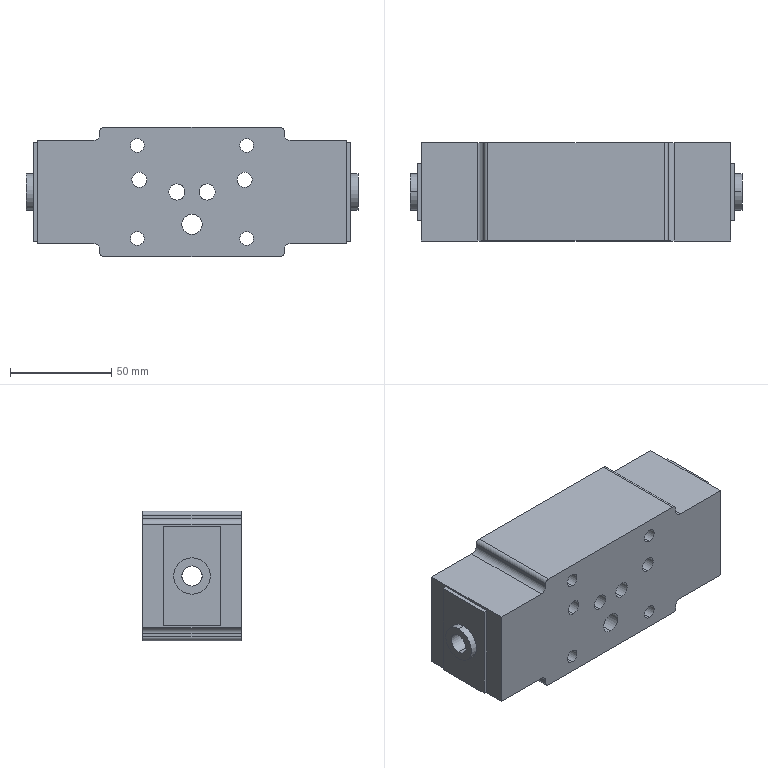Part | SolidWorks | features ICE 4, Extrusion 1, MirrorPattern 1 | 1 solid | 62 faces | box 164 x 48.5 x 64 mm | volume 411589 mm3 | cylinder 36 | plane 26 | commonest cylinder face diameters 6.8 x8 8 x8 4 x4 6 x4 7.5 x4 10 x4